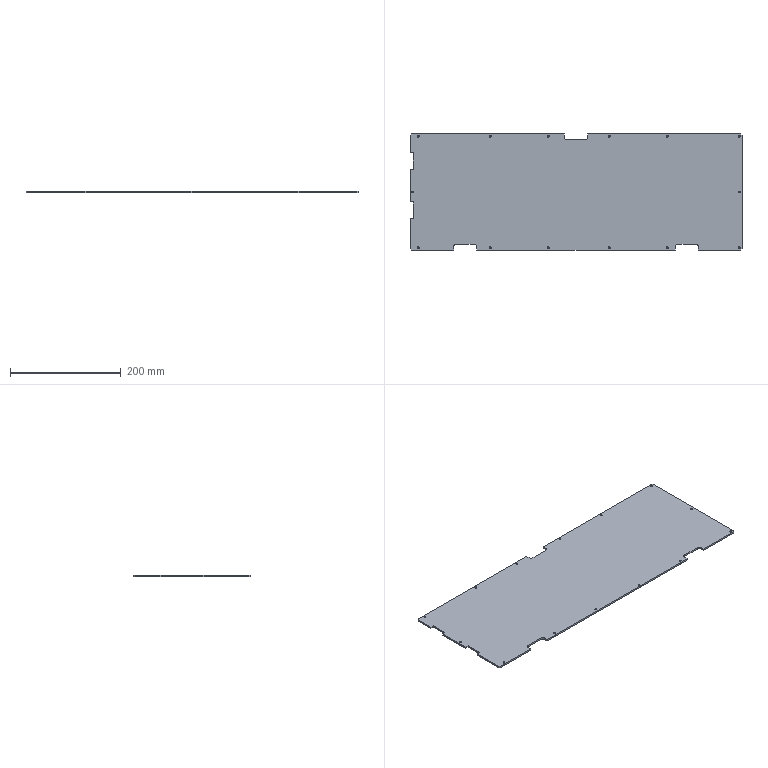Part | SolidWorks | features Chamfer 2, ICE 2, Cut 1, Extrusion 1, Fillet 1, MoveFace 1 | 1 solid | 92 faces | box 600 x 210 x 3 mm | volume 372208 mm3 | cylinder 34 | plane 30 | cone 28 | commonest cylinder face diameters 3.5 x28 10 x6